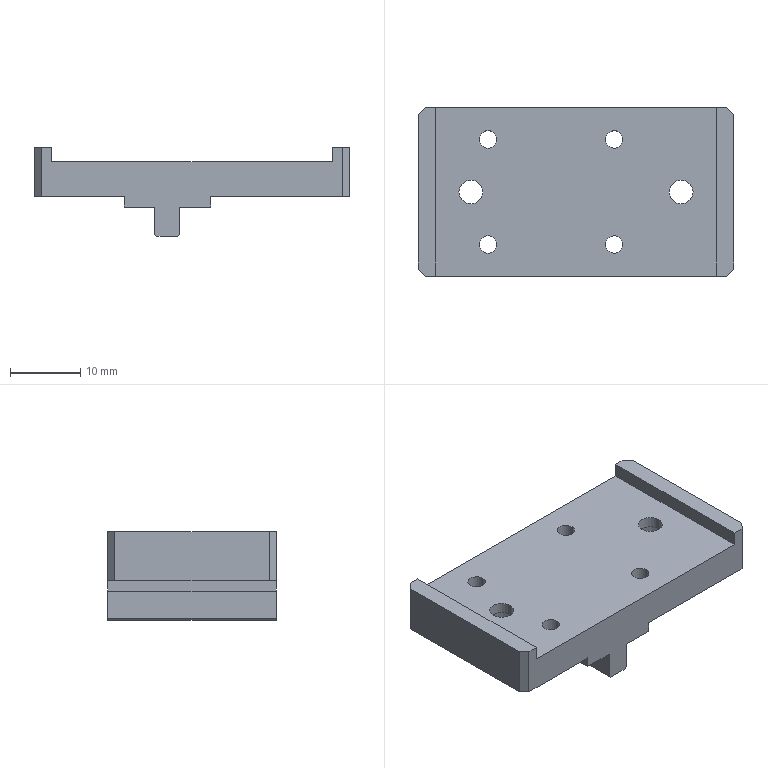Part | STEP file | PN_0039 | 1 solid | 42 faces | box 45 x 24 x 12.7 mm | volume 6100 mm3 | plane 26 | cylinder 16 | commonest cylinder face diameters 2.5 x8 3.4 x4 6 x4